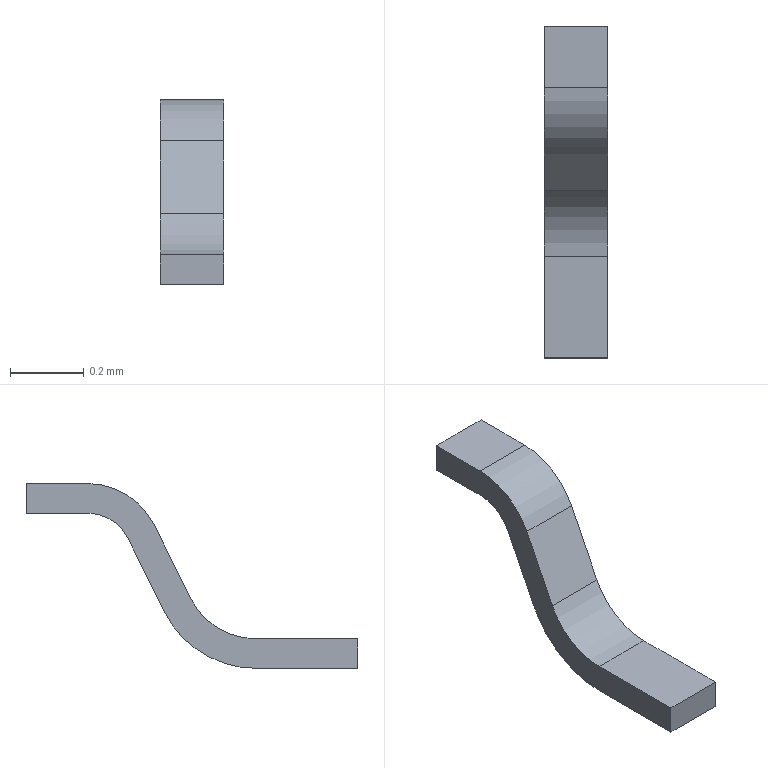Part | STEP file | RJ-USIO-V1_2-220411_29 | 1 solid | 15 faces | box 0.1708 x 0.8974 x 0.5 mm | volume 0.01511 mm3 | plane 11 | cylinder 4 | commonest cylinder face diameters 0.4 x2 0.24 x1 0.56 x1